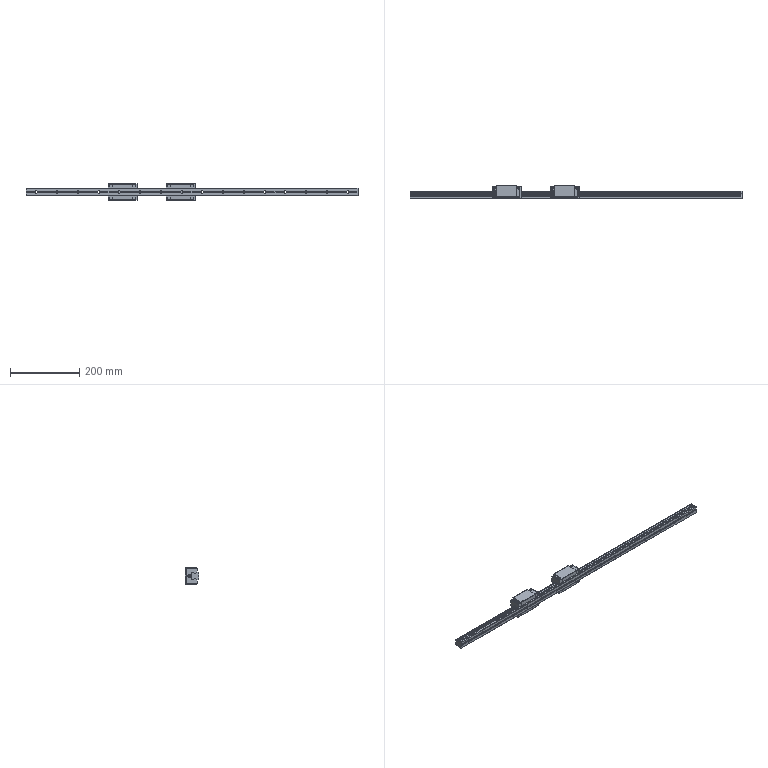Part | SolidWorks | 11 solids | 1373 faces | box 960 x 40 x 48 mm | volume 597195 mm3 | plane 924 | cylinder 368 | spline 57 | cone 24 | commonest cylinder face diameters 0.24 x51 2 x44 4.6 x44 7 x32 11 x32 0.12 x27